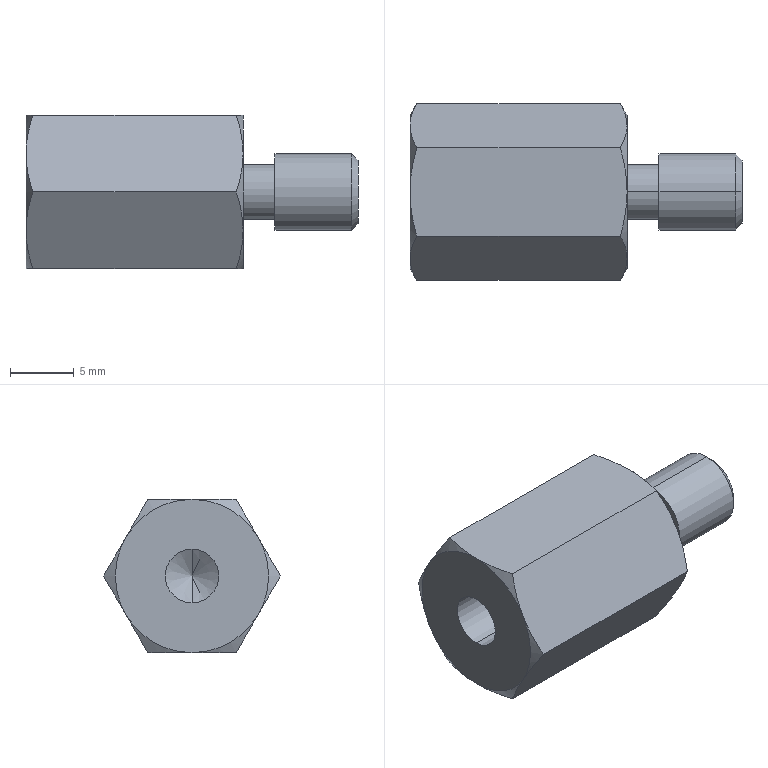Part | STEP file | 0228_215_Post | 1 solid | 32 faces | box 26 x 13.856 x 12 mm | volume 2134 mm3 | cone 16 | plane 10 | cylinder 6 | commonest cylinder face diameters 4.2 x2 4.3 x2 6 x2